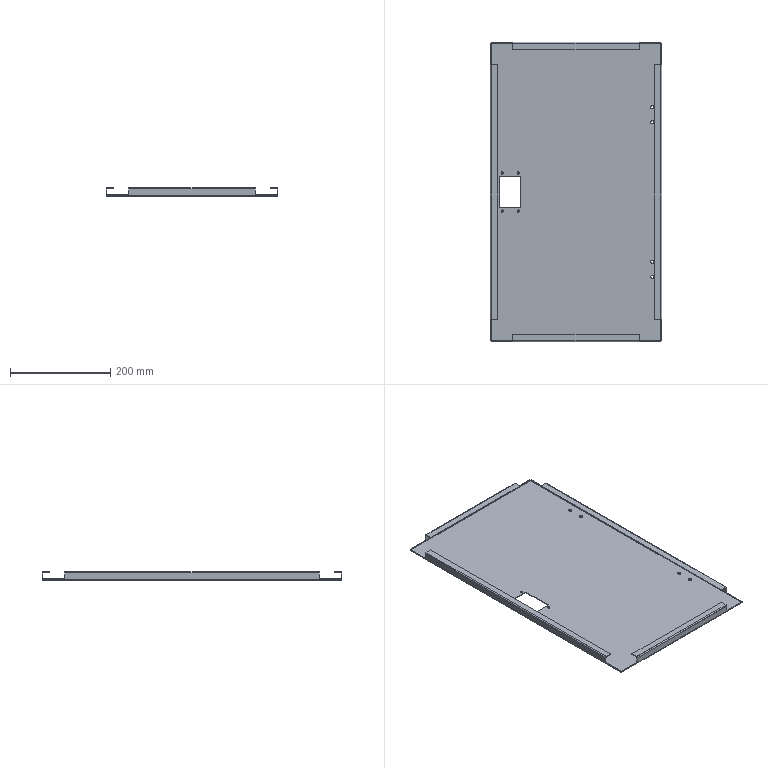Part | SolidWorks | features BaseBody 1 | 1 solid | 106 faces | box 342.5 x 598 x 16.5 mm | volume 365126 mm3 | plane 66 | cylinder 32 | spline 8 | commonest cylinder face diameters 1.473 x8 4.473 x8 4.5 x8 6.6 x8